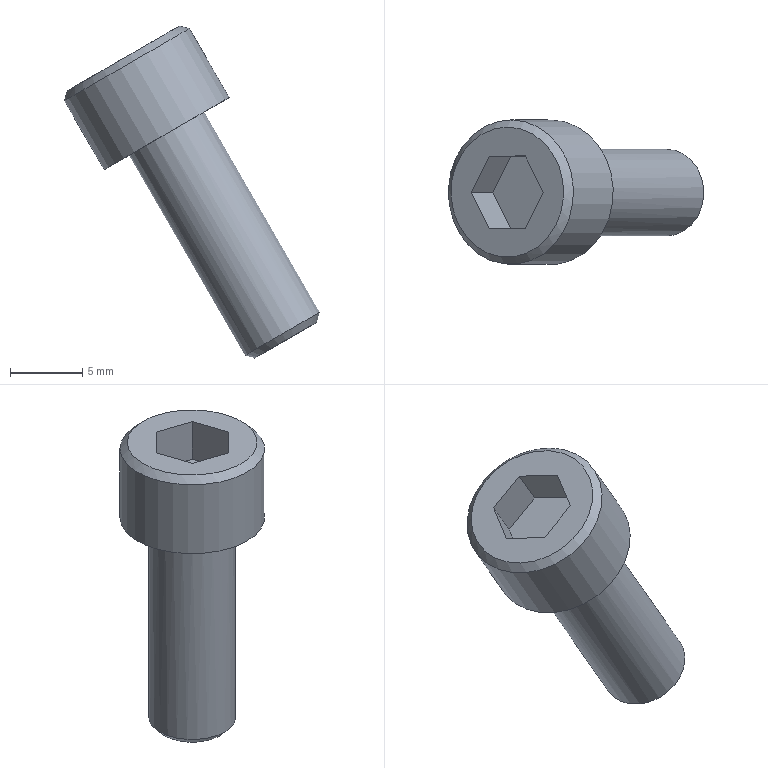Part | STEP file | solid 3 | 1 solid | 14 faces | box 17.678 x 10 x 22.986 mm | volume 866.792 mm3 | plane 10 | cone 2 | cylinder 2 | commonest cylinder face diameters 6 x1 10 x1